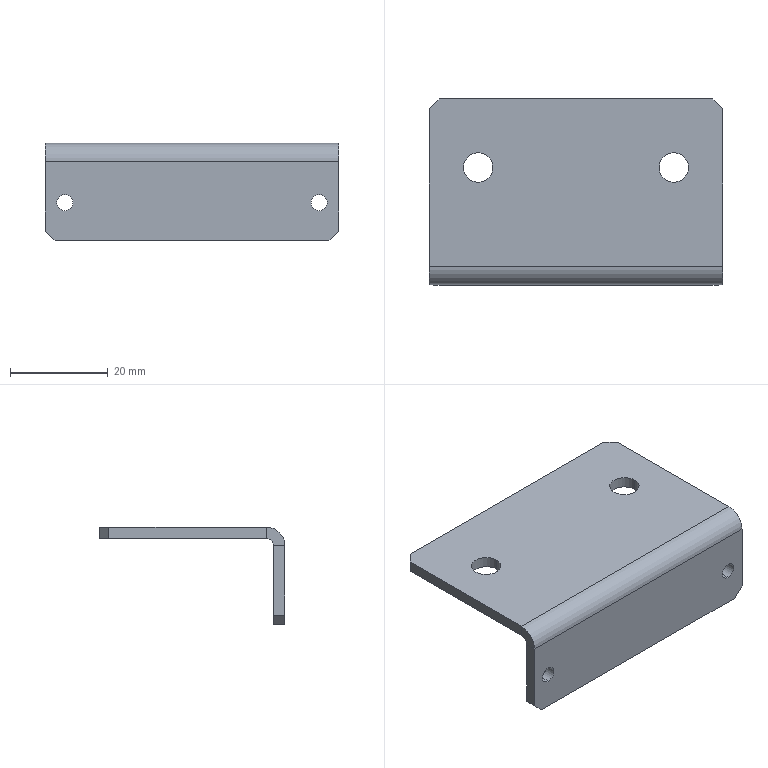Part | STEP file | 227H056122 Sensor BKT_Default | 1 solid | 26 faces | box 60 x 38 x 20 mm | volume 7342 mm3 | plane 16 | cylinder 10 | commonest cylinder face diameters 3.3 x4 6 x4 3 x1 7.6 x1